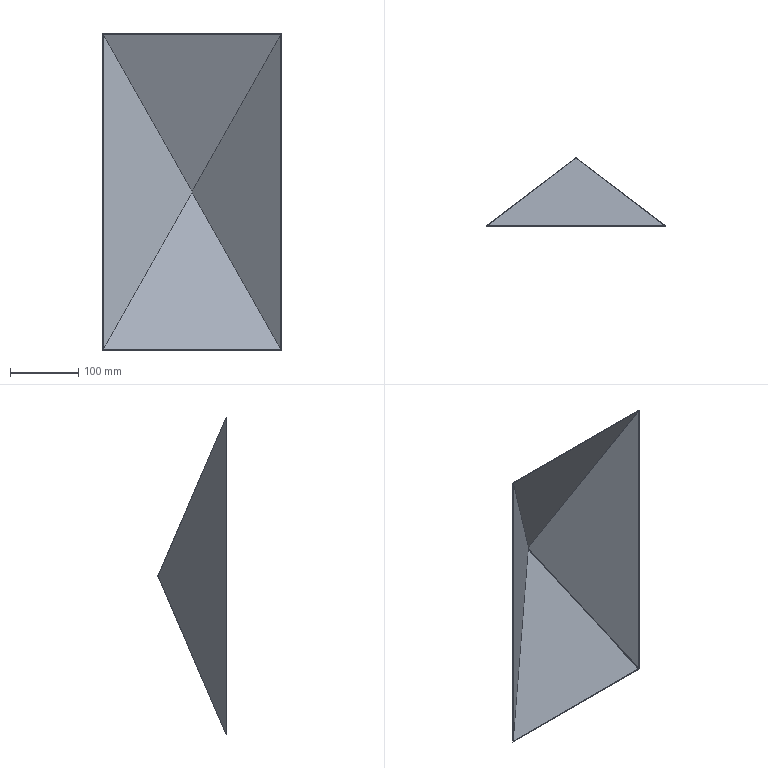Part | SolidWorks | features 3DProfileFeature 5, CirPattern 2, FillRefSurface 2, Thicken 2, RefAxis 1 | 2 solids | 26 faces | box 263.013 x 100 x 465.513 mm | volume 119004 mm3 | plane 26
STEP:
#1=CARTESIAN_POINT('',(1.,0.,0.));
#2=VERTEX_POINT('',#1);
#3=CARTESIAN_POINT('',(0.5,-0.3802,0.885));
#4=VERTEX_POINT('',#3);
#5=CARTESIAN_POINT('',(-130.507,-100.,232.756));
#6=DIRECTION('',(-0.4607,-0.3504,0.8155));
#7=VECTOR('',#6,1000.);
#8=LINE('',#5,#7);
#9=EDGE_CURVE('',#2,#4,#8,.T.);
#10=ORIENTED_EDGE('',*,*,#9,.T.);
#11=CARTESIAN_POINT('',(0.5,-0.3802,-0.885));
#12=VERTEX_POINT('',#11);
#13=CARTESIAN_POINT('',(0.5,-0.3802,0.));
#14=DIRECTION('',(0.,0.,-1.));
#15=VECTOR('',#14,1000.);
#16=LINE('',#13,#15);
#17=EDGE_CURVE('',#4,#12,#16,.T.);
#18=ORIENTED_EDGE('',*,*,#17,.T.);
#19=CARTESIAN_POINT('',(1.,0.,0.));
#20=DIRECTION('',(0.4607,0.3504,0.8155));
#21=VECTOR('',#20,1000.);
#22=LINE('',#19,#21);
#23=EDGE_CURVE('',#12,#2,#22,.T.);
#24=ORIENTED_EDGE('',*,*,#23,.T.);
#25=EDGE_LOOP('',(#10,#18,#24));
#26=FACE_OUTER_BOUND('',#25,.T.);
#27=CARTESIAN_POINT('',(1.,0.,0.));
#28=DIRECTION('',(0.6053,-0.796,0.));
#29=DIRECTION('',(0.796,0.6053,0.));
#30=AXIS2_PLACEMENT_3D('',#27,#28,#29);
#31=PLANE('',#30);
#32=ADVANCED_FACE('',(#26),#31,.T.);
#33=CARTESIAN_POINT('',(-0.2825,-0.2148,0.5));
#34=VERTEX_POINT('',#33);
#35=CARTESIAN_POINT('',(0.,0.,0.));
#36=VERTEX_POINT('',#35);
#37=CARTESIAN_POINT('',(0.,0.,0.));
#38=DIRECTION('',(0.4607,0.3504,-0.8155));
#39=VECTOR('',#38,1000.);
#40=LINE('',#37,#39);
#41=EDGE_CURVE('',#34,#36,#40,.T.);
#42=ORIENTED_EDGE('',*,*,#41,.F.);
#43=CARTESIAN_POINT('',(0.,0.,1.));
#44=VERTEX_POINT('',#43);
#45=CARTESIAN_POINT('',(0.,0.,1.));
#46=DIRECTION('',(-0.4607,-0.3504,-0.8155));
#47=VECTOR('',#46,1000.);
#48=LINE('',#45,#47);
#49=EDGE_CURVE('',#44,#34,#48,.T.);
#50=ORIENTED_EDGE('',*,*,#49,.F.);
#51=CARTESIAN_POINT('',(0.,0.,1.));
#52=CARTESIAN_POINT('',(0.,0.,0.6667));
#53=CARTESIAN_POINT('',(0.,0.,0.3333));
#54=CARTESIAN_POINT('',(0.,0.,0.));
#55=B_SPLINE_CURVE_WITH_KNOTS('',3,(#51,#52,#53,#54),.UNSPECIFIED.,.F.,.F.,(4,4),(0.,1.),.UNSPECIFIED.);
#56=EDGE_CURVE('',#44,#36,#55,.T.);
#57=ORIENTED_EDGE('',*,*,#56,.T.);
#58=EDGE_LOOP('',(#42,#50,#57));
#59=FACE_OUTER_BOUND('',#58,.T.);
#60=CARTESIAN_POINT('',(0.,0.,0.));
#61=DIRECTION('',(0.6053,-0.796,0.));
#62=DIRECTION('',(0.796,0.6053,0.));
#63=AXIS2_PLACEMENT_3D('',#60,#61,#62);
#64=PLANE('',#63);
#65=ADVANCED_FACE('',(#59),#64,.F.);
#66=CARTESIAN_POINT('',(0.,-0.7604,1.77));
#67=VERTEX_POINT('',#66);
#68=CARTESIAN_POINT('',(-130.507,-100.,232.756));
#69=VERTEX_POINT('',#68);
#70=CARTESIAN_POINT('',(-130.507,-100.,232.756));
#71=DIRECTION('',(-0.4607,-0.3504,0.8155));
#72=VECTOR('',#71,1000.);
#73=LINE('',#70,#72);
#74=EDGE_CURVE('',#67,#69,#73,.T.);
#75=ORIENTED_EDGE('',*,*,#74,.F.);
#76=CARTESIAN_POINT('',(130.507,-100.,232.756));
#77=VERTEX_POINT('',#76);
#78=CARTESIAN_POINT('',(-1.,0.,0.));
#79=DIRECTION('',(-0.4607,0.3504,-0.8155));
#80=VECTOR('',#79,1000.);
#81=LINE('',#78,#80);
#82=EDGE_CURVE('',#77,#67,#81,.T.);
#83=ORIENTED_EDGE('',*,*,#82,.F.);
#84=CARTESIAN_POINT('',(131.507,-100.,232.756));
#85=VERTEX_POINT('',#84);
#86=CARTESIAN_POINT('',(130.507,-100.,232.756));
#87=CARTESIAN_POINT('',(130.84,-100.,232.756));
#88=CARTESIAN_POINT('',(131.173,-100.,232.756));
#89=CARTESIAN_POINT('',(131.507,-100.,232.756));
#90=B_SPLINE_CURVE_WITH_KNOTS('',3,(#86,#87,#88,#89),.UNSPECIFIED.,.F.,.F.,(4,4),(0.,1.),.UNSPECIFIED.);
#91=EDGE_CURVE('',#77,#85,#90,.T.);
#92=ORIENTED_EDGE('',*,*,#91,.T.);
#93=CARTESIAN_POINT('',(0.,0.,0.));
#94=DIRECTION('',(-0.4607,0.3504,-0.8155));
#95=VECTOR('',#94,1000.);
#96=LINE('',#93,#95);
#97=EDGE_CURVE('',#85,#4,#96,.T.);
#98=ORIENTED_EDGE('',*,*,#97,.T.);
#99=ORIENTED_EDGE('',*,*,#9,.F.);
#100=CARTESIAN_POINT('',(1.,0.,0.));
#101=CARTESIAN_POINT('',(0.6667,0.,0.));
#102=CARTESIAN_POINT('',(0.3333,0.,0.));
#103=CARTESIAN_POINT('',(0.,0.,0.));
#104=B_SPLINE_CURVE_WITH_KNOTS('',3,(#100,#101,#102,#103),.UNSPECIFIED.,.F.,.F.,(4,4),(0.,1.),.UNSPECIFIED.);
#105=EDGE_CURVE('',#2,#36,#104,.T.);
#106=ORIENTED_EDGE('',*,*,#105,.T.);
#107=CARTESIAN_POINT('',(0.2825,-0.2148,0.5));
#108=VERTEX_POINT('',#107);
#109=CARTESIAN_POINT('',(75.888,-57.706,134.315));
#110=DIRECTION('',(-0.4607,0.3504,-0.8155));
#111=VECTOR('',#110,1000.);
#112=LINE('',#109,#111);
#113=EDGE_CURVE('',#108,#36,#112,.T.);
#114=ORIENTED_EDGE('',*,*,#113,.F.);
#115=CARTESIAN_POINT('',(-130.507,-0.2148,0.5));
#116=DIRECTION('',(-1.,0.,0.));
#117=VECTOR('',#116,1000.);
#118=LINE('',#115,#117);
#119=EDGE_CURVE('',#108,#34,#118,.T.);
#120=ORIENTED_EDGE('',*,*,#119,.T.);
#121=ORIENTED_EDGE('',*,*,#41,.T.);
#122=CARTESIAN_POINT('',(-1.,0.,0.));
#123=VERTEX_POINT('',#122);
#124=CARTESIAN_POINT('',(-1.,0.,0.));
#125=CARTESIAN_POINT('',(-0.6667,0.,0.));
#126=CARTESIAN_POINT('',(-0.3333,0.,0.));
#127=CARTESIAN_POINT('',(0.,0.,0.));
#128=B_SPLINE_CURVE_WITH_KNOTS('',3,(#124,#125,#126,#127),.UNSPECIFIED.,.F.,.F.,(4,4),(0.,1.),.UNSPECIFIED.);
#129=EDGE_CURVE('',#123,#36,#128,.T.);
#130=ORIENTED_EDGE('',*,*,#129,.F.);
#131=CARTESIAN_POINT('',(-0.5,-0.3802,0.885));
#132=VERTEX_POINT('',#131);
#133=CARTESIAN_POINT('',(-1.,0.,0.));
#134=DIRECTION('',(-0.4607,0.3504,-0.8155));
#135=VECTOR('',#134,1000.);
#136=LINE('',#133,#135);
#137=EDGE_CURVE('',#132,#123,#136,.T.);
#138=ORIENTED_EDGE('',*,*,#137,.F.);
#139=CARTESIAN_POINT('',(-131.507,-100.,232.756));
#140=VERTEX_POINT('',#139);
#141=CARTESIAN_POINT('',(-131.507,-100.,232.756));
#142=DIRECTION('',(-0.4607,-0.3504,0.8155));
#143=VECTOR('',#142,1000.);
#144=LINE('',#141,#143);
#145=EDGE_CURVE('',#132,#140,#144,.T.);
#146=ORIENTED_EDGE('',*,*,#145,.T.);
#147=CARTESIAN_POINT('',(-130.507,-100.,232.756));
#148=CARTESIAN_POINT('',(-130.84,-100.,232.756));
#149=CARTESIAN_POINT('',(-131.173,-100.,232.756));
#150=CARTESIAN_POINT('',(-131.507,-100.,232.756));
#151=B_SPLINE_CURVE_WITH_KNOTS('',3,(#147,#148,#149,#150),.UNSPECIFIED.,.F.,.F.,(4,4),(0.,1.),.UNSPECIFIED.);
#152=EDGE_CURVE('',#69,#140,#151,.T.);
#153=ORIENTED_EDGE('',*,*,#152,.F.);
#154=EDGE_LOOP('',(#75,#83,#92,#98,#99,#106,#114,#120,#121,#130,#138,#146,#153));
#155=FACE_OUTER_BOUND('',#154,.T.);
#156=CARTESIAN_POINT('',(-130.507,-100.,232.756));
#157=DIRECTION('',(0.,-0.9188,-0.3947));
#158=DIRECTION('',(0.,0.3947,-0.9188));
#159=AXIS2_PLACEMENT_3D('',#156,#157,#158);
#160=PLANE('',#159);
#161=ADVANCED_FACE('',(#155),#160,.F.);
#162=CARTESIAN_POINT('',(0.,-0.7604,-0.7699));
#163=VERTEX_POINT('',#162);
#164=CARTESIAN_POINT('',(0.,-0.7604,0.));
#165=DIRECTION('',(0.,0.,-1.));
#166=VECTOR('',#165,1000.);
#167=LINE('',#164,#166);
#168=EDGE_CURVE('',#67,#163,#167,.T.);
#169=ORIENTED_EDGE('',*,*,#168,.F.);
#170=ORIENTED_EDGE('',*,*,#74,.T.);
#171=CARTESIAN_POINT('',(-130.507,-100.,-231.756));
#172=VERTEX_POINT('',#171);
#173=CARTESIAN_POINT('',(-130.507,-100.,232.756));
#174=DIRECTION('',(0.,0.,-1.));
#175=VECTOR('',#174,1000.);
#176=LINE('',#173,#175);
#177=EDGE_CURVE('',#69,#172,#176,.T.);
#178=ORIENTED_EDGE('',*,*,#177,.T.);
#179=CARTESIAN_POINT('',(0.6243,-0.2857,0.335));
#180=DIRECTION('',(-0.4607,-0.3504,-0.8155));
#181=VECTOR('',#180,1000.);
#182=LINE('',#179,#181);
#183=EDGE_CURVE('',#163,#172,#182,.T.);
#184=ORIENTED_EDGE('',*,*,#183,.F.);
#185=EDGE_LOOP('',(#169,#170,#178,#184));
#186=FACE_OUTER_BOUND('',#185,.T.);
#187=CARTESIAN_POINT('',(1.,0.,0.));
#188=DIRECTION('',(0.6053,-0.796,0.));
#189=DIRECTION('',(0.796,0.6053,0.));
#190=AXIS2_PLACEMENT_3D('',#187,#188,#189);
#191=PLANE('',#190);
#192=ADVANCED_FACE('',(#186),#191,.T.);
#193=CARTESIAN_POINT('',(-131.507,-100.,-232.756));
#194=VERTEX_POINT('',#193);
#195=CARTESIAN_POINT('',(-0.5,-0.3802,-0.885));
#196=VERTEX_POINT('',#195);
#197=CARTESIAN_POINT('',(0.,0.,0.));
#198=DIRECTION('',(0.4607,0.3504,0.8155));
#199=VECTOR('',#198,1000.);
#200=LINE('',#197,#199);
#201=EDGE_CURVE('',#194,#196,#200,.T.);
#202=ORIENTED_EDGE('',*,*,#201,.T.);
#203=CARTESIAN_POINT('',(130.507,-100.,-232.756));
#204=DIRECTION('',(0.4607,-0.3504,-0.8155));
#205=VECTOR('',#204,1000.);
#206=LINE('',#203,#205);
#207=EDGE_CURVE('',#123,#196,#206,.T.);
#208=ORIENTED_EDGE('',*,*,#207,.F.);
#209=ORIENTED_EDGE('',*,*,#129,.T.);
#210=ORIENTED_EDGE('',*,*,#105,.F.);
#211=ORIENTED_EDGE('',*,*,#23,.F.);
#212=CARTESIAN_POINT('',(131.507,-100.,-232.756));
#213=VERTEX_POINT('',#212);
#214=CARTESIAN_POINT('',(131.507,-100.,-232.756));
#215=DIRECTION('',(-0.4607,0.3504,0.8155));
#216=VECTOR('',#215,1000.);
#217=LINE('',#214,#216);
#218=EDGE_CURVE('',#213,#12,#217,.T.);
#219=ORIENTED_EDGE('',*,*,#218,.F.);
#220=CARTESIAN_POINT('',(-130.507,-100.,-232.756));
#221=VERTEX_POINT('',#220);
#222=CARTESIAN_POINT('',(-131.507,-100.,-232.756));
#223=DIRECTION('',(1.,0.,0.));
#224=VECTOR('',#223,1000.);
#225=LINE('',#222,#224);
#226=EDGE_CURVE('',#221,#213,#225,.T.);
#227=ORIENTED_EDGE('',*,*,#226,.F.);
#228=CARTESIAN_POINT('',(-130.507,-100.,-232.756));
#229=CARTESIAN_POINT('',(-130.84,-100.,-232.756));
#230=CARTESIAN_POINT('',(-131.173,-100.,-232.756));
#231=CARTESIAN_POINT('',(-131.507,-100.,-232.756));
#232=B_SPLINE_CURVE_WITH_KNOTS('',3,(#228,#229,#230,#231),.UNSPECIFIED.,.F.,.F.,(4,4),(0.,1.),.UNSPECIFIED.);
#233=EDGE_CURVE('',#221,#194,#232,.T.);
#234=ORIENTED_EDGE('',*,*,#233,.T.);
#235=EDGE_LOOP('',(#202,#208,#209,#210,#211,#219,#227,#234));
#236=FACE_OUTER_BOUND('',#235,.T.);
#237=CARTESIAN_POINT('',(1.,0.,0.));
#238=DIRECTION('',(0.,-0.9188,0.3947));
#239=DIRECTION('',(0.,-0.3947,-0.9188));
#240=AXIS2_PLACEMENT_3D('',#237,#238,#239);
#241=PLANE('',#240);
#242=ADVANCED_FACE('',(#236),#241,.F.);
#243=ORIENTED_EDGE('',*,*,#226,.T.);
#244=CARTESIAN_POINT('',(131.507,-100.,-231.756));
#245=VERTEX_POINT('',#244);
#246=CARTESIAN_POINT('',(131.507,-100.,-231.756));
#247=CARTESIAN_POINT('',(131.507,-100.,-232.09));
#248=CARTESIAN_POINT('',(131.507,-100.,-232.423));
#249=CARTESIAN_POINT('',(131.507,-100.,-232.756));
#250=B_SPLINE_CURVE_WITH_KNOTS('',3,(#246,#247,#248,#249),.UNSPECIFIED.,.F.,.F.,(4,4),(0.,1.),.UNSPECIFIED.);
#251=EDGE_CURVE('',#245,#213,#250,.T.);
#252=ORIENTED_EDGE('',*,*,#251,.F.);
#253=CARTESIAN_POINT('',(131.507,-100.,-232.756));
#254=DIRECTION('',(0.,0.,1.));
#255=VECTOR('',#254,1000.);
#256=LINE('',#253,#255);
#257=EDGE_CURVE('',#245,#85,#256,.T.);
#258=ORIENTED_EDGE('',*,*,#257,.T.);
#259=ORIENTED_EDGE('',*,*,#91,.F.);
#260=CARTESIAN_POINT('',(130.507,-100.,-231.756));
#261=VERTEX_POINT('',#260);
#262=CARTESIAN_POINT('',(130.507,-100.,-232.756));
#263=DIRECTION('',(0.,0.,1.));
#264=VECTOR('',#263,1000.);
#265=LINE('',#262,#264);
#266=EDGE_CURVE('',#261,#77,#265,.T.);
#267=ORIENTED_EDGE('',*,*,#266,.F.);
#268=CARTESIAN_POINT('',(-131.507,-100.,-231.756));
#269=DIRECTION('',(1.,0.,0.));
#270=VECTOR('',#269,1000.);
#271=LINE('',#268,#270);
#272=EDGE_CURVE('',#172,#261,#271,.T.);
#273=ORIENTED_EDGE('',*,*,#272,.F.);
#274=ORIENTED_EDGE('',*,*,#177,.F.);
#275=ORIENTED_EDGE('',*,*,#152,.T.);
#276=CARTESIAN_POINT('',(-131.507,-100.,232.756));
#277=DIRECTION('',(0.,0.,-1.));
#278=VECTOR('',#277,1000.);
#279=LINE('',#276,#278);
#280=EDGE_CURVE('',#140,#194,#279,.T.);
#281=ORIENTED_EDGE('',*,*,#280,.T.);
#282=ORIENTED_EDGE('',*,*,#233,.F.);
#283=EDGE_LOOP('',(#243,#252,#258,#259,#267,#273,#274,#275,#281,#282));
#284=FACE_OUTER_BOUND('',#283,.T.);
#285=CARTESIAN_POINT('',(-130.507,-100.,232.756));
#286=DIRECTION('',(0.,1.,0.));
#287=DIRECTION('',(0.,0.,1.));
#288=AXIS2_PLACEMENT_3D('',#285,#286,#287);
#289=PLANE('',#288);
#290=ADVANCED_FACE('',(#284),#289,.F.);
#291=ORIENTED_EDGE('',*,*,#145,.F.);
#292=CARTESIAN_POINT('',(-0.5,-0.3802,0.));
#293=DIRECTION('',(0.,0.,-1.));
#294=VECTOR('',#293,1000.);
#295=LINE('',#292,#294);
#296=EDGE_CURVE('',#132,#196,#295,.T.);
#297=ORIENTED_EDGE('',*,*,#296,.T.);
#298=ORIENTED_EDGE('',*,*,#201,.F.);
#299=ORIENTED_EDGE('',*,*,#280,.F.);
#300=EDGE_LOOP('',(#291,#297,#298,#299));
#301=FACE_OUTER_BOUND('',#300,.T.);
#302=CARTESIAN_POINT('',(0.,0.,0.));
#303=DIRECTION('',(0.6053,-0.796,0.));
#304=DIRECTION('',(0.796,0.6053,0.));
#305=AXIS2_PLACEMENT_3D('',#302,#303,#304);
#306=PLANE('',#305);
#307=ADVANCED_FACE('',(#301),#306,.F.);
#308=CARTESIAN_POINT('',(-0.7877,-0.1614,0.6243));
#309=DIRECTION('',(0.4607,-0.3504,-0.8155));
#310=VECTOR('',#309,1000.);
#311=LINE('',#308,#310);
#312=EDGE_CURVE('',#163,#261,#311,.T.);
#313=ORIENTED_EDGE('',*,*,#312,.F.);
#314=ORIENTED_EDGE('',*,*,#183,.T.);
#315=ORIENTED_EDGE('',*,*,#272,.T.);
#316=EDGE_LOOP('',(#313,#314,#315));
#317=FACE_OUTER_BOUND('',#316,.T.);
#318=CARTESIAN_POINT('',(0.,0.,1.));
#319=DIRECTION('',(0.,-0.9188,0.3947));
#320=DIRECTION('',(0.,-0.3947,-0.9188));
#321=AXIS2_PLACEMENT_3D('',#318,#319,#320);
#322=PLANE('',#321);
#323=ADVANCED_FACE('',(#317),#322,.T.);
#324=ORIENTED_EDGE('',*,*,#17,.F.);
#325=ORIENTED_EDGE('',*,*,#97,.F.);
#326=ORIENTED_EDGE('',*,*,#257,.F.);
#327=ORIENTED_EDGE('',*,*,#251,.T.);
#328=ORIENTED_EDGE('',*,*,#218,.T.);
#329=EDGE_LOOP('',(#324,#325,#326,#327,#328));
#330=FACE_OUTER_BOUND('',#329,.T.);
#331=CARTESIAN_POINT('',(131.507,-100.,-231.756));
#332=DIRECTION('',(-0.6053,-0.796,0.));
#333=DIRECTION('',(0.796,-0.6053,0.));
#334=AXIS2_PLACEMENT_3D('',#331,#332,#333);
#335=PLANE('',#334);
#336=ADVANCED_FACE('',(#330),#335,.F.);
#337=CARTESIAN_POINT('',(131.507,-100.,-231.756));
#338=DIRECTION('',(-0.4607,0.3504,0.8155));
#339=VECTOR('',#338,1000.);
#340=LINE('',#337,#339);
#341=EDGE_CURVE('',#108,#44,#340,.T.);
#342=ORIENTED_EDGE('',*,*,#341,.F.);
#343=ORIENTED_EDGE('',*,*,#113,.T.);
#344=ORIENTED_EDGE('',*,*,#56,.F.);
#345=EDGE_LOOP('',(#342,#343,#344));
#346=FACE_OUTER_BOUND('',#345,.T.);
#347=CARTESIAN_POINT('',(131.507,-100.,-231.756));
#348=DIRECTION('',(-0.6053,-0.796,0.));
#349=DIRECTION('',(0.796,-0.6053,0.));
#350=AXIS2_PLACEMENT_3D('',#347,#348,#349);
#351=PLANE('',#350);
#352=ADVANCED_FACE('',(#346),#351,.F.);
#353=ORIENTED_EDGE('',*,*,#119,.F.);
#354=ORIENTED_EDGE('',*,*,#341,.T.);
#355=ORIENTED_EDGE('',*,*,#49,.T.);
#356=EDGE_LOOP('',(#353,#354,#355));
#357=FACE_OUTER_BOUND('',#356,.T.);
#358=CARTESIAN_POINT('',(0.,0.,1.));
#359=DIRECTION('',(0.,-0.9188,0.3947));
#360=DIRECTION('',(0.,-0.3947,-0.9188));
#361=AXIS2_PLACEMENT_3D('',#358,#359,#360);
#362=PLANE('',#361);
#363=ADVANCED_FACE('',(#357),#362,.T.);
#364=ORIENTED_EDGE('',*,*,#82,.T.);
#365=ORIENTED_EDGE('',*,*,#168,.T.);
#366=ORIENTED_EDGE('',*,*,#312,.T.);
#367=ORIENTED_EDGE('',*,*,#266,.T.);
#368=EDGE_LOOP('',(#364,#365,#366,#367));
#369=FACE_OUTER_BOUND('',#368,.T.);
#370=CARTESIAN_POINT('',(-1.,0.,0.));
#371=DIRECTION('',(-0.6053,-0.796,0.));
#372=DIRECTION('',(-0.796,0.6053,0.));
#373=AXIS2_PLACEMENT_3D('',#370,#371,#372);
#374=PLANE('',#373);
#375=ADVANCED_FACE('',(#369),#374,.T.);
#376=ORIENTED_EDGE('',*,*,#296,.F.);
#377=ORIENTED_EDGE('',*,*,#137,.T.);
#378=ORIENTED_EDGE('',*,*,#207,.T.);
#379=EDGE_LOOP('',(#376,#377,#378));
#380=FACE_OUTER_BOUND('',#379,.T.);
#381=CARTESIAN_POINT('',(-1.,0.,0.));
#382=DIRECTION('',(-0.6053,-0.796,0.));
#383=DIRECTION('',(-0.796,0.6053,0.));
#384=AXIS2_PLACEMENT_3D('',#381,#382,#383);
#385=PLANE('',#384);
#386=ADVANCED_FACE('',(#380),#385,.T.);
#387=CLOSED_SHELL('',(#32,#65,#161,#192,#242,#290,#307,#323,#336,#352,#363,#375,#386));
#388=MANIFOLD_SOLID_BREP('',#387);
#389=CARTESIAN_POINT('',(-1.,0.,0.));
#390=VERTEX_POINT('',#389);
#391=CARTESIAN_POINT('',(-0.5,-0.3802,-0.885));
#392=VERTEX_POINT('',#391);
#393=CARTESIAN_POINT('',(130.507,-100.,-232.756));
#394=DIRECTION('',(0.4607,-0.3504,-0.8155));
#395=VECTOR('',#394,1000.);
#396=LINE('',#393,#395);
#397=EDGE_CURVE('',#390,#392,#396,.T.);
#398=ORIENTED_EDGE('',*,*,#397,.T.);
#399=CARTESIAN_POINT('',(-0.5,-0.3802,0.885));
#400=VERTEX_POINT('',#399);
#401=CARTESIAN_POINT('',(-0.5,-0.3802,0.));
#402=DIRECTION('',(0.,0.,1.));
#403=VECTOR('',#402,1000.);
#404=LINE('',#401,#403);
#405=EDGE_CURVE('',#392,#400,#404,.T.);
#406=ORIENTED_EDGE('',*,*,#405,.T.);
#407=CARTESIAN_POINT('',(-1.,0.,0.));
#408=DIRECTION('',(-0.4607,0.3504,-0.8155));
#409=VECTOR('',#408,1000.);
#410=LINE('',#407,#409);
#411=EDGE_CURVE('',#400,#390,#410,.T.);
#412=ORIENTED_EDGE('',*,*,#411,.T.);
#413=EDGE_LOOP('',(#398,#406,#412));
#414=FACE_OUTER_BOUND('',#413,.T.);
#415=CARTESIAN_POINT('',(-1.,0.,0.));
#416=DIRECTION('',(-0.6053,-0.796,0.));
#417=DIRECTION('',(-0.796,0.6053,0.));
#418=AXIS2_PLACEMENT_3D('',#415,#416,#417);
#419=PLANE('',#418);
#420=ADVANCED_FACE('',(#414),#419,.T.);
#421=CARTESIAN_POINT('',(0.2825,-0.2148,-0.5));
#422=VERTEX_POINT('',#421);
#423=CARTESIAN_POINT('',(0.,0.,0.));
#424=VERTEX_POINT('',#423);
#425=CARTESIAN_POINT('',(0.,0.,0.));
#426=DIRECTION('',(-0.4607,0.3504,0.8155));
#427=VECTOR('',#426,1000.);
#428=LINE('',#425,#427);
#429=EDGE_CURVE('',#422,#424,#428,.T.);
#430=ORIENTED_EDGE('',*,*,#429,.F.);
#431=CARTESIAN_POINT('',(0.,0.,-1.));
#432=VERTEX_POINT('',#431);
#433=CARTESIAN_POINT('',(0.,0.,-1.));
#434=DIRECTION('',(0.4607,-0.3504,0.8155));
#435=VECTOR('',#434,1000.);
#436=LINE('',#433,#435);
#437=EDGE_CURVE('',#432,#422,#436,.T.);
#438=ORIENTED_EDGE('',*,*,#437,.F.);
#439=CARTESIAN_POINT('',(0.,0.,-1.));
#440=CARTESIAN_POINT('',(0.,0.,-0.6667));
#441=CARTESIAN_POINT('',(0.,0.,-0.3333));
#442=CARTESIAN_POINT('',(0.,0.,0.));
#443=B_SPLINE_CURVE_WITH_KNOTS('',3,(#439,#440,#441,#442),.UNSPECIFIED.,.F.,.F.,(4,4),(0.,1.),.UNSPECIFIED.);
#444=EDGE_CURVE('',#432,#424,#443,.T.);
#445=ORIENTED_EDGE('',*,*,#444,.T.);
#446=EDGE_LOOP('',(#430,#438,#445));
#447=FACE_OUTER_BOUND('',#446,.T.);
#448=CARTESIAN_POINT('',(0.,0.,0.));
#449=DIRECTION('',(-0.6053,-0.796,0.));
#450=DIRECTION('',(-0.796,0.6053,0.));
#451=AXIS2_PLACEMENT_3D('',#448,#449,#450);
#452=PLANE('',#451);
#453=ADVANCED_FACE('',(#447),#452,.F.);
#454=CARTESIAN_POINT('',(0.,-0.7604,-1.77));
#455=VERTEX_POINT('',#454);
#456=CARTESIAN_POINT('',(130.507,-100.,-232.756));
#457=VERTEX_POINT('',#456);
#458=CARTESIAN_POINT('',(130.507,-100.,-232.756));
#459=DIRECTION('',(0.4607,-0.3504,-0.8155));
#460=VECTOR('',#459,1000.);
#461=LINE('',#458,#460);
#462=EDGE_CURVE('',#455,#457,#461,.T.);
#463=ORIENTED_EDGE('',*,*,#462,.F.);
#464=CARTESIAN_POINT('',(-130.507,-100.,-232.756));
#465=VERTEX_POINT('',#464);
#466=CARTESIAN_POINT('',(1.,0.,0.));
#467=DIRECTION('',(0.4607,0.3504,0.8155));
#468=VECTOR('',#467,1000.);
#469=LINE('',#466,#468);
#470=EDGE_CURVE('',#465,#455,#469,.T.);
#471=ORIENTED_EDGE('',*,*,#470,.F.);
#472=CARTESIAN_POINT('',(-131.507,-100.,-232.756));
#473=VERTEX_POINT('',#472);
#474=CARTESIAN_POINT('',(-130.507,-100.,-232.756));
#475=CARTESIAN_POINT('',(-130.84,-100.,-232.756));
#476=CARTESIAN_POINT('',(-131.173,-100.,-232.756));
#477=CARTESIAN_POINT('',(-131.507,-100.,-232.756));
#478=B_SPLINE_CURVE_WITH_KNOTS('',3,(#474,#475,#476,#477),.UNSPECIFIED.,.F.,.F.,(4,4),(0.,1.),.UNSPECIFIED.);
#479=EDGE_CURVE('',#465,#473,#478,.T.);
#480=ORIENTED_EDGE('',*,*,#479,.T.);
#481=CARTESIAN_POINT('',(0.,0.,0.));
#482=DIRECTION('',(0.4607,0.3504,0.8155));
#483=VECTOR('',#482,1000.);
#484=LINE('',#481,#483);
#485=EDGE_CURVE('',#473,#392,#484,.T.);
#486=ORIENTED_EDGE('',*,*,#485,.T.);
#487=ORIENTED_EDGE('',*,*,#397,.F.);
#488=CARTESIAN_POINT('',(-1.,0.,0.));
#489=CARTESIAN_POINT('',(-0.6667,0.,0.));
#490=CARTESIAN_POINT('',(-0.3333,0.,0.));
#491=CARTESIAN_POINT('',(0.,0.,0.));
#492=B_SPLINE_CURVE_WITH_KNOTS('',3,(#488,#489,#490,#491),.UNSPECIFIED.,.F.,.F.,(4,4),(0.,1.),.UNSPECIFIED.);
#493=EDGE_CURVE('',#390,#424,#492,.T.);
#494=ORIENTED_EDGE('',*,*,#493,.T.);
#495=CARTESIAN_POINT('',(-0.2825,-0.2148,-0.5));
#496=VERTEX_POINT('',#495);
#497=CARTESIAN_POINT('',(-75.888,-57.706,-134.315));
#498=DIRECTION('',(0.4607,0.3504,0.8155));
#499=VECTOR('',#498,1000.);
#500=LINE('',#497,#499);
#501=EDGE_CURVE('',#496,#424,#500,.T.);
#502=ORIENTED_EDGE('',*,*,#501,.F.);
#503=CARTESIAN_POINT('',(130.507,-0.2148,-0.5));
#504=DIRECTION('',(1.,0.,0.));
#505=VECTOR('',#504,1000.);
#506=LINE('',#503,#505);
#507=EDGE_CURVE('',#496,#422,#506,.T.);
#508=ORIENTED_EDGE('',*,*,#507,.T.);
#509=ORIENTED_EDGE('',*,*,#429,.T.);
#510=CARTESIAN_POINT('',(1.,0.,0.));
#511=VERTEX_POINT('',#510);
#512=CARTESIAN_POINT('',(1.,0.,0.));
#513=CARTESIAN_POINT('',(0.6667,0.,0.));
#514=CARTESIAN_POINT('',(0.3333,0.,0.));
#515=CARTESIAN_POINT('',(0.,0.,0.));
#516=B_SPLINE_CURVE_WITH_KNOTS('',3,(#512,#513,#514,#515),.UNSPECIFIED.,.F.,.F.,(4,4),(0.,1.),.UNSPECIFIED.);
#517=EDGE_CURVE('',#511,#424,#516,.T.);
#518=ORIENTED_EDGE('',*,*,#517,.F.);
#519=CARTESIAN_POINT('',(0.5,-0.3802,-0.885));
#520=VERTEX_POINT('',#519);
#521=CARTESIAN_POINT('',(1.,0.,0.));
#522=DIRECTION('',(0.4607,0.3504,0.8155));
#523=VECTOR('',#522,1000.);
#524=LINE('',#521,#523);
#525=EDGE_CURVE('',#520,#511,#524,.T.);
#526=ORIENTED_EDGE('',*,*,#525,.F.);
#527=CARTESIAN_POINT('',(131.507,-100.,-232.756));
#528=VERTEX_POINT('',#527);
#529=CARTESIAN_POINT('',(131.507,-100.,-232.756));
#530=DIRECTION('',(0.4607,-0.3504,-0.8155));
#531=VECTOR('',#530,1000.);
#532=LINE('',#529,#531);
#533=EDGE_CURVE('',#520,#528,#532,.T.);
#534=ORIENTED_EDGE('',*,*,#533,.T.);
#535=CARTESIAN_POINT('',(130.507,-100.,-232.756));
#536=CARTESIAN_POINT('',(130.84,-100.,-232.756));
#537=CARTESIAN_POINT('',(131.173,-100.,-232.756));
#538=CARTESIAN_POINT('',(131.507,-100.,-232.756));
#539=B_SPLINE_CURVE_WITH_KNOTS('',3,(#535,#536,#537,#538),.UNSPECIFIED.,.F.,.F.,(4,4),(0.,1.),.UNSPECIFIED.);
#540=EDGE_CURVE('',#457,#528,#539,.T.);
#541=ORIENTED_EDGE('',*,*,#540,.F.);
#542=EDGE_LOOP('',(#463,#471,#480,#486,#487,#494,#502,#508,#509,#518,#526,#534,#541));
#543=FACE_OUTER_BOUND('',#542,.T.);
#544=CARTESIAN_POINT('',(130.507,-100.,-232.756));
#545=DIRECTION('',(0.,-0.9188,0.3947));
#546=DIRECTION('',(0.,0.3947,0.9188));
#547=AXIS2_PLACEMENT_3D('',#544,#545,#546);
#548=PLANE('',#547);
#549=ADVANCED_FACE('',(#543),#548,.F.);
#550=CARTESIAN_POINT('',(0.,-0.7604,0.7699));
#551=VERTEX_POINT('',#550);
#552=CARTESIAN_POINT('',(0.,-0.7604,0.));
#553=DIRECTION('',(0.,0.,1.));
#554=VECTOR('',#553,1000.);
#555=LINE('',#552,#554);
#556=EDGE_CURVE('',#455,#551,#555,.T.);
#557=ORIENTED_EDGE('',*,*,#556,.F.);
#558=ORIENTED_EDGE('',*,*,#462,.T.);
#559=CARTESIAN_POINT('',(130.507,-100.,231.756));
#560=VERTEX_POINT('',#559);
#561=CARTESIAN_POINT('',(130.507,-100.,-232.756));
#562=DIRECTION('',(0.,0.,1.));
#563=VECTOR('',#562,1000.);
#564=LINE('',#561,#563);
#565=EDGE_CURVE('',#457,#560,#564,.T.);
#566=ORIENTED_EDGE('',*,*,#565,.T.);
#567=CARTESIAN_POINT('',(-0.6243,-0.2857,-0.335));
#568=DIRECTION('',(0.4607,-0.3504,0.8155));
#569=VECTOR('',#568,1000.);
#570=LINE('',#567,#569);
#571=EDGE_CURVE('',#551,#560,#570,.T.);
#572=ORIENTED_EDGE('',*,*,#571,.F.);
#573=EDGE_LOOP('',(#557,#558,#566,#572));
#574=FACE_OUTER_BOUND('',#573,.T.);
#575=CARTESIAN_POINT('',(-1.,0.,0.));
#576=DIRECTION('',(-0.6053,-0.796,0.));
#577=DIRECTION('',(-0.796,0.6053,0.));
#578=AXIS2_PLACEMENT_3D('',#575,#576,#577);
#579=PLANE('',#578);
#580=ADVANCED_FACE('',(#574),#579,.T.);
#581=CARTESIAN_POINT('',(131.507,-100.,232.756));
#582=VERTEX_POINT('',#581);
#583=CARTESIAN_POINT('',(0.5,-0.3802,0.885));
#584=VERTEX_POINT('',#583);
#585=CARTESIAN_POINT('',(0.,0.,0.));
#586=DIRECTION('',(-0.4607,0.3504,-0.8155));
#587=VECTOR('',#586,1000.);
#588=LINE('',#585,#587);
#589=EDGE_CURVE('',#582,#584,#588,.T.);
#590=ORIENTED_EDGE('',*,*,#589,.T.);
#591=CARTESIAN_POINT('',(-130.507,-100.,232.756));
#592=DIRECTION('',(-0.4607,-0.3504,0.8155));
#593=VECTOR('',#592,1000.);
#594=LINE('',#591,#593);
#595=EDGE_CURVE('',#511,#584,#594,.T.);
#596=ORIENTED_EDGE('',*,*,#595,.F.);
#597=ORIENTED_EDGE('',*,*,#517,.T.);
#598=ORIENTED_EDGE('',*,*,#493,.F.);
#599=ORIENTED_EDGE('',*,*,#411,.F.);
#600=CARTESIAN_POINT('',(-131.507,-100.,232.756));
#601=VERTEX_POINT('',#600);
#602=CARTESIAN_POINT('',(-131.507,-100.,232.756));
#603=DIRECTION('',(0.4607,0.3504,-0.8155));
#604=VECTOR('',#603,1000.);
#605=LINE('',#602,#604);
#606=EDGE_CURVE('',#601,#400,#605,.T.);
#607=ORIENTED_EDGE('',*,*,#606,.F.);
#608=CARTESIAN_POINT('',(130.507,-100.,232.756));
#609=VERTEX_POINT('',#608);
#610=CARTESIAN_POINT('',(131.507,-100.,232.756));
#611=DIRECTION('',(-1.,0.,0.));
#612=VECTOR('',#611,1000.);
#613=LINE('',#610,#612);
#614=EDGE_CURVE('',#609,#601,#613,.T.);
#615=ORIENTED_EDGE('',*,*,#614,.F.);
#616=CARTESIAN_POINT('',(130.507,-100.,232.756));
#617=CARTESIAN_POINT('',(130.84,-100.,232.756));
#618=CARTESIAN_POINT('',(131.173,-100.,232.756));
#619=CARTESIAN_POINT('',(131.507,-100.,232.756));
#620=B_SPLINE_CURVE_WITH_KNOTS('',3,(#616,#617,#618,#619),.UNSPECIFIED.,.F.,.F.,(4,4),(0.,1.),.UNSPECIFIED.);
#621=EDGE_CURVE('',#609,#582,#620,.T.);
#622=ORIENTED_EDGE('',*,*,#621,.T.);
#623=EDGE_LOOP('',(#590,#596,#597,#598,#599,#607,#615,#622));
#624=FACE_OUTER_BOUND('',#623,.T.);
#625=CARTESIAN_POINT('',(-1.,0.,0.));
#626=DIRECTION('',(0.,-0.9188,-0.3947));
#627=DIRECTION('',(0.,-0.3947,0.9188));
#628=AXIS2_PLACEMENT_3D('',#625,#626,#627);
#629=PLANE('',#628);
#630=ADVANCED_FACE('',(#624),#629,.F.);
#631=ORIENTED_EDGE('',*,*,#614,.T.);
#632=CARTESIAN_POINT('',(-131.507,-100.,231.756));
#633=VERTEX_POINT('',#632);
#634=CARTESIAN_POINT('',(-131.507,-100.,231.756));
#635=CARTESIAN_POINT('',(-131.507,-100.,232.09));
#636=CARTESIAN_POINT('',(-131.507,-100.,232.423));
#637=CARTESIAN_POINT('',(-131.507,-100.,232.756));
#638=B_SPLINE_CURVE_WITH_KNOTS('',3,(#634,#635,#636,#637),.UNSPECIFIED.,.F.,.F.,(4,4),(0.,1.),.UNSPECIFIED.);
#639=EDGE_CURVE('',#633,#601,#638,.T.);
#640=ORIENTED_EDGE('',*,*,#639,.F.);
#641=CARTESIAN_POINT('',(-131.507,-100.,232.756));
#642=DIRECTION('',(0.,0.,-1.));
#643=VECTOR('',#642,1000.);
#644=LINE('',#641,#643);
#645=EDGE_CURVE('',#633,#473,#644,.T.);
#646=ORIENTED_EDGE('',*,*,#645,.T.);
#647=ORIENTED_EDGE('',*,*,#479,.F.);
#648=CARTESIAN_POINT('',(-130.507,-100.,231.756));
#649=VERTEX_POINT('',#648);
#650=CARTESIAN_POINT('',(-130.507,-100.,232.756));
#651=DIRECTION('',(0.,0.,-1.));
#652=VECTOR('',#651,1000.);
#653=LINE('',#650,#652);
#654=EDGE_CURVE('',#649,#465,#653,.T.);
#655=ORIENTED_EDGE('',*,*,#654,.F.);
#656=CARTESIAN_POINT('',(131.507,-100.,231.756));
#657=DIRECTION('',(-1.,0.,0.));
#658=VECTOR('',#657,1000.);
#659=LINE('',#656,#658);
#660=EDGE_CURVE('',#560,#649,#659,.T.);
#661=ORIENTED_EDGE('',*,*,#660,.F.);
#662=ORIENTED_EDGE('',*,*,#565,.F.);
#663=ORIENTED_EDGE('',*,*,#540,.T.);
#664=CARTESIAN_POINT('',(131.507,-100.,-232.756));
#665=DIRECTION('',(0.,0.,1.));
#666=VECTOR('',#665,1000.);
#667=LINE('',#664,#666);
#668=EDGE_CURVE('',#528,#582,#667,.T.);
#669=ORIENTED_EDGE('',*,*,#668,.T.);
#670=ORIENTED_EDGE('',*,*,#621,.F.);
#671=EDGE_LOOP('',(#631,#640,#646,#647,#655,#661,#662,#663,#669,#670));
#672=FACE_OUTER_BOUND('',#671,.T.);
#673=CARTESIAN_POINT('',(130.507,-100.,-232.756));
#674=DIRECTION('',(0.,1.,0.));
#675=DIRECTION('',(0.,0.,-1.));
#676=AXIS2_PLACEMENT_3D('',#673,#674,#675);
#677=PLANE('',#676);
#678=ADVANCED_FACE('',(#672),#677,.F.);
#679=ORIENTED_EDGE('',*,*,#533,.F.);
#680=CARTESIAN_POINT('',(0.5,-0.3802,0.));
#681=DIRECTION('',(0.,0.,1.));
#682=VECTOR('',#681,1000.);
#683=LINE('',#680,#682);
#684=EDGE_CURVE('',#520,#584,#683,.T.);
#685=ORIENTED_EDGE('',*,*,#684,.T.);
#686=ORIENTED_EDGE('',*,*,#589,.F.);
#687=ORIENTED_EDGE('',*,*,#668,.F.);
#688=EDGE_LOOP('',(#679,#685,#686,#687));
#689=FACE_OUTER_BOUND('',#688,.T.);
#690=CARTESIAN_POINT('',(0.,0.,0.));
#691=DIRECTION('',(-0.6053,-0.796,0.));
#692=DIRECTION('',(-0.796,0.6053,0.));
#693=AXIS2_PLACEMENT_3D('',#690,#691,#692);
#694=PLANE('',#693);
#695=ADVANCED_FACE('',(#689),#694,.F.);
#696=CARTESIAN_POINT('',(0.7877,-0.1614,-0.6243));
#697=DIRECTION('',(-0.4607,-0.3504,0.8155));
#698=VECTOR('',#697,1000.);
#699=LINE('',#696,#698);
#700=EDGE_CURVE('',#551,#649,#699,.T.);
#701=ORIENTED_EDGE('',*,*,#700,.F.);
#702=ORIENTED_EDGE('',*,*,#571,.T.);
#703=ORIENTED_EDGE('',*,*,#660,.T.);
#704=EDGE_LOOP('',(#701,#702,#703));
#705=FACE_OUTER_BOUND('',#704,.T.);
#706=CARTESIAN_POINT('',(0.,0.,-1.));
#707=DIRECTION('',(0.,-0.9188,-0.3947));
#708=DIRECTION('',(0.,-0.3947,0.9188));
#709=AXIS2_PLACEMENT_3D('',#706,#707,#708);
#710=PLANE('',#709);
#711=ADVANCED_FACE('',(#705),#710,.T.);
#712=ORIENTED_EDGE('',*,*,#405,.F.);
#713=ORIENTED_EDGE('',*,*,#485,.F.);
#714=ORIENTED_EDGE('',*,*,#645,.F.);
#715=ORIENTED_EDGE('',*,*,#639,.T.);
#716=ORIENTED_EDGE('',*,*,#606,.T.);
#717=EDGE_LOOP('',(#712,#713,#714,#715,#716));
#718=FACE_OUTER_BOUND('',#717,.T.);
#719=CARTESIAN_POINT('',(-131.507,-100.,231.756));
#720=DIRECTION('',(0.6053,-0.796,0.));
#721=DIRECTION('',(-0.796,-0.6053,0.));
#722=AXIS2_PLACEMENT_3D('',#719,#720,#721);
#723=PLANE('',#722);
#724=ADVANCED_FACE('',(#718),#723,.F.);
#725=CARTESIAN_POINT('',(-131.507,-100.,231.756));
#726=DIRECTION('',(0.4607,0.3504,-0.8155));
#727=VECTOR('',#726,1000.);
#728=LINE('',#725,#727);
#729=EDGE_CURVE('',#496,#432,#728,.T.);
#730=ORIENTED_EDGE('',*,*,#729,.F.);
#731=ORIENTED_EDGE('',*,*,#501,.T.);
#732=ORIENTED_EDGE('',*,*,#444,.F.);
#733=EDGE_LOOP('',(#730,#731,#732));
#734=FACE_OUTER_BOUND('',#733,.T.);
#735=CARTESIAN_POINT('',(-131.507,-100.,231.756));
#736=DIRECTION('',(0.6053,-0.796,0.));
#737=DIRECTION('',(-0.796,-0.6053,0.));
#738=AXIS2_PLACEMENT_3D('',#735,#736,#737);
#739=PLANE('',#738);
#740=ADVANCED_FACE('',(#734),#739,.F.);
#741=ORIENTED_EDGE('',*,*,#507,.F.);
#742=ORIENTED_EDGE('',*,*,#729,.T.);
#743=ORIENTED_EDGE('',*,*,#437,.T.);
#744=EDGE_LOOP('',(#741,#742,#743));
#745=FACE_OUTER_BOUND('',#744,.T.);
#746=CARTESIAN_POINT('',(0.,0.,-1.));
#747=DIRECTION('',(0.,-0.9188,-0.3947));
#748=DIRECTION('',(0.,-0.3947,0.9188));
#749=AXIS2_PLACEMENT_3D('',#746,#747,#748);
#750=PLANE('',#749);
#751=ADVANCED_FACE('',(#745),#750,.T.);
#752=ORIENTED_EDGE('',*,*,#470,.T.);
#753=ORIENTED_EDGE('',*,*,#556,.T.);
#754=ORIENTED_EDGE('',*,*,#700,.T.);
#755=ORIENTED_EDGE('',*,*,#654,.T.);
#756=EDGE_LOOP('',(#752,#753,#754,#755));
#757=FACE_OUTER_BOUND('',#756,.T.);
#758=CARTESIAN_POINT('',(1.,0.,0.));
#759=DIRECTION('',(0.6053,-0.796,0.));
#760=DIRECTION('',(0.796,0.6053,0.));
#761=AXIS2_PLACEMENT_3D('',#758,#759,#760);
#762=PLANE('',#761);
#763=ADVANCED_FACE('',(#757),#762,.T.);
#764=ORIENTED_EDGE('',*,*,#684,.F.);
#765=ORIENTED_EDGE('',*,*,#525,.T.);
#766=ORIENTED_EDGE('',*,*,#595,.T.);
#767=EDGE_LOOP('',(#764,#765,#766));
#768=FACE_OUTER_BOUND('',#767,.T.);
#769=CARTESIAN_POINT('',(1.,0.,0.));
#770=DIRECTION('',(0.6053,-0.796,0.));
#771=DIRECTION('',(0.796,0.6053,0.));
#772=AXIS2_PLACEMENT_3D('',#769,#770,#771);
#773=PLANE('',#772);
#774=ADVANCED_FACE('',(#768),#773,.T.);
#775=CLOSED_SHELL('',(#420,#453,#549,#580,#630,#678,#695,#711,#724,#740,#751,#763,#774));
#776=MANIFOLD_SOLID_BREP('',#775);
#777=CARTESIAN_POINT('',(0.,0.,0.));
#778=DIRECTION('',(0.,0.,1.));
#779=DIRECTION('',(1.,0.,0.));
#780=AXIS2_PLACEMENT_3D('',#777,#778,#779);
#781=(LENGTH_UNIT()NAMED_UNIT(*)SI_UNIT(.MILLI.,.METRE.));
#782=UNCERTAINTY_MEASURE_WITH_UNIT(LENGTH_MEASURE(0.00001),#781,'','');
#783=(NAMED_UNIT(*)PLANE_ANGLE_UNIT()SI_UNIT($,.RADIAN.));
#784=(NAMED_UNIT(*)SI_UNIT($,.STERADIAN.)SOLID_ANGLE_UNIT());
#785=(GEOMETRIC_REPRESENTATION_CONTEXT(3)GLOBAL_UNCERTAINTY_ASSIGNED_CONTEXT((#782))GLOBAL_UNIT_ASSIGNED_CONTEXT((#781,#783,#784))REPRESENTATION_CONTEXT('',''));
#786=ADVANCED_BREP_SHAPE_REPRESENTATION('',(#388,#776,#780),#785);